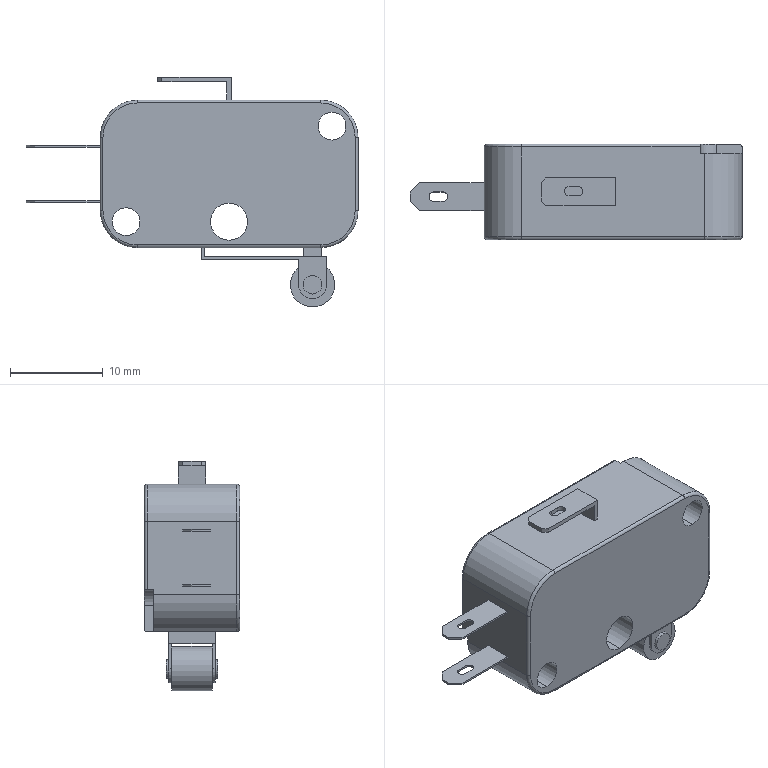Part | STEP file | V-155-1C25 | 1 solid | 104 faces | box 35.8 x 10.3 x 24.8 mm | volume 4254 mm3 | plane 60 | cylinder 38 | torus 6 | commonest cylinder face diameters 1 x9 0.6 x8 3 x7 2 x4 8 x4 4 x2